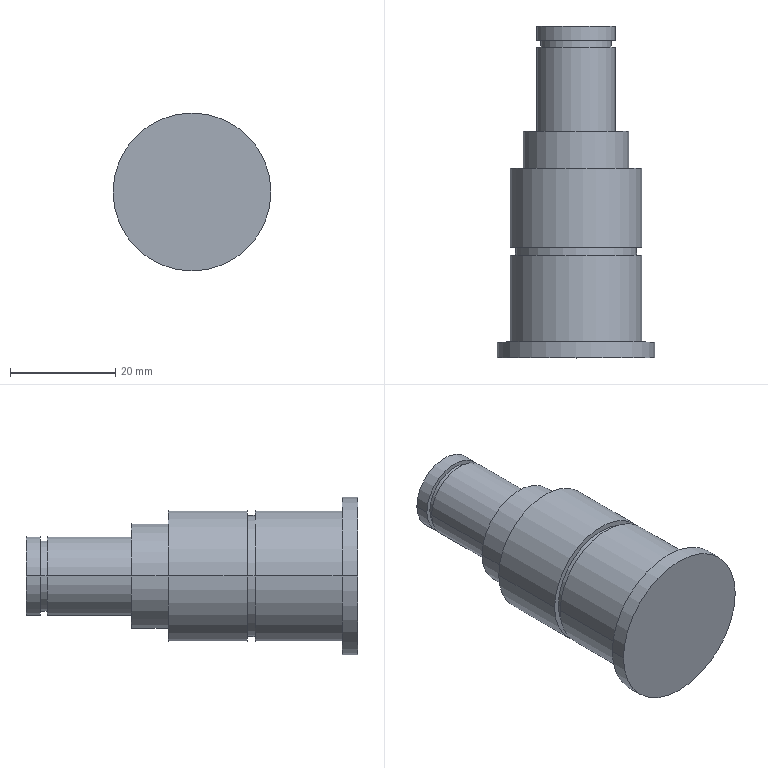Part | SolidWorks | features Revolution 1 | 1 solid | 25 faces | box 30 x 63 x 30 mm | volume 23893 mm3 | cylinder 16 | plane 9 | commonest cylinder face diameters 15 x4 25 x4 13.4 x2 20 x2 23 x2 30 x2
STEP:
#1=CARTESIAN_POINT('',(6.7,63.005,0.));
#2=VERTEX_POINT('',#1);
#3=CARTESIAN_POINT('',(-6.7,63.005,0.));
#4=VERTEX_POINT('',#3);
#5=CARTESIAN_POINT('',(0.,63.005,0.));
#6=DIRECTION('',(0.,-1.,0.));
#7=DIRECTION('',(1.,0.,0.));
#8=AXIS2_PLACEMENT_3D('',#5,#6,#7);
#9=CIRCLE('',#8,6.7);
#10=EDGE_CURVE('',#2,#4,#9,.T.);
#11=ORIENTED_EDGE('',*,*,#10,.T.);
#12=CARTESIAN_POINT('',(-6.7,61.705,0.));
#13=VERTEX_POINT('',#12);
#14=CARTESIAN_POINT('',(-6.7,65.705,0.));
#15=DIRECTION('',(0.,-1.,0.));
#16=VECTOR('',#15,1000.);
#17=LINE('',#14,#16);
#18=EDGE_CURVE('',#4,#13,#17,.T.);
#19=ORIENTED_EDGE('',*,*,#18,.T.);
#20=CARTESIAN_POINT('',(6.7,61.705,0.));
#21=VERTEX_POINT('',#20);
#22=CARTESIAN_POINT('',(0.,61.705,0.));
#23=DIRECTION('',(0.,-1.,0.));
#24=DIRECTION('',(1.,0.,0.));
#25=AXIS2_PLACEMENT_3D('',#22,#23,#24);
#26=CIRCLE('',#25,6.7);
#27=EDGE_CURVE('',#21,#13,#26,.T.);
#28=ORIENTED_EDGE('',*,*,#27,.F.);
#29=CARTESIAN_POINT('',(6.7,65.705,0.));
#30=DIRECTION('',(0.,-1.,0.));
#31=VECTOR('',#30,1000.);
#32=LINE('',#29,#31);
#33=EDGE_CURVE('',#2,#21,#32,.T.);
#34=ORIENTED_EDGE('',*,*,#33,.F.);
#35=EDGE_LOOP('',(#11,#19,#28,#34));
#36=FACE_OUTER_BOUND('',#35,.T.);
#37=CARTESIAN_POINT('',(0.,65.705,0.));
#38=DIRECTION('',(0.,-1.,0.));
#39=DIRECTION('',(1.,0.,0.));
#40=AXIS2_PLACEMENT_3D('',#37,#38,#39);
#41=CYLINDRICAL_SURFACE('',#40,6.7);
#42=ADVANCED_FACE('',(#36),#41,.T.);
#43=CARTESIAN_POINT('',(7.5,61.705,0.));
#44=VERTEX_POINT('',#43);
#45=CARTESIAN_POINT('',(-7.5,61.705,0.));
#46=VERTEX_POINT('',#45);
#47=CARTESIAN_POINT('',(0.,61.705,0.));
#48=DIRECTION('',(0.,-1.,0.));
#49=DIRECTION('',(1.,0.,0.));
#50=AXIS2_PLACEMENT_3D('',#47,#48,#49);
#51=CIRCLE('',#50,7.5);
#52=EDGE_CURVE('',#44,#46,#51,.T.);
#53=ORIENTED_EDGE('',*,*,#52,.T.);
#54=CARTESIAN_POINT('',(-7.5,45.705,0.));
#55=VERTEX_POINT('',#54);
#56=CARTESIAN_POINT('',(-7.5,65.705,0.));
#57=DIRECTION('',(0.,-1.,0.));
#58=VECTOR('',#57,1000.);
#59=LINE('',#56,#58);
#60=EDGE_CURVE('',#46,#55,#59,.T.);
#61=ORIENTED_EDGE('',*,*,#60,.T.);
#62=CARTESIAN_POINT('',(7.5,45.705,0.));
#63=VERTEX_POINT('',#62);
#64=CARTESIAN_POINT('',(0.,45.705,0.));
#65=DIRECTION('',(0.,-1.,0.));
#66=DIRECTION('',(1.,0.,0.));
#67=AXIS2_PLACEMENT_3D('',#64,#65,#66);
#68=CIRCLE('',#67,7.5);
#69=EDGE_CURVE('',#63,#55,#68,.T.);
#70=ORIENTED_EDGE('',*,*,#69,.F.);
#71=CARTESIAN_POINT('',(7.5,65.705,0.));
#72=DIRECTION('',(0.,-1.,0.));
#73=VECTOR('',#72,1000.);
#74=LINE('',#71,#73);
#75=EDGE_CURVE('',#44,#63,#74,.T.);
#76=ORIENTED_EDGE('',*,*,#75,.F.);
#77=EDGE_LOOP('',(#53,#61,#70,#76));
#78=FACE_OUTER_BOUND('',#77,.T.);
#79=CARTESIAN_POINT('',(0.,65.705,0.));
#80=DIRECTION('',(0.,-1.,0.));
#81=DIRECTION('',(1.,0.,0.));
#82=AXIS2_PLACEMENT_3D('',#79,#80,#81);
#83=CYLINDRICAL_SURFACE('',#82,7.5);
#84=ADVANCED_FACE('',(#78),#83,.T.);
#85=CARTESIAN_POINT('',(10.,45.705,0.));
#86=VERTEX_POINT('',#85);
#87=CARTESIAN_POINT('',(-10.,45.705,0.));
#88=VERTEX_POINT('',#87);
#89=CARTESIAN_POINT('',(0.,45.705,0.));
#90=DIRECTION('',(0.,-1.,0.));
#91=DIRECTION('',(1.,0.,0.));
#92=AXIS2_PLACEMENT_3D('',#89,#90,#91);
#93=CIRCLE('',#92,10.);
#94=EDGE_CURVE('',#86,#88,#93,.T.);
#95=ORIENTED_EDGE('',*,*,#94,.T.);
#96=CARTESIAN_POINT('',(-10.,38.705,0.));
#97=VERTEX_POINT('',#96);
#98=CARTESIAN_POINT('',(-10.,65.705,0.));
#99=DIRECTION('',(0.,-1.,0.));
#100=VECTOR('',#99,1000.);
#101=LINE('',#98,#100);
#102=EDGE_CURVE('',#88,#97,#101,.T.);
#103=ORIENTED_EDGE('',*,*,#102,.T.);
#104=CARTESIAN_POINT('',(10.,38.705,0.));
#105=VERTEX_POINT('',#104);
#106=CARTESIAN_POINT('',(0.,38.705,0.));
#107=DIRECTION('',(0.,-1.,0.));
#108=DIRECTION('',(1.,0.,0.));
#109=AXIS2_PLACEMENT_3D('',#106,#107,#108);
#110=CIRCLE('',#109,10.);
#111=EDGE_CURVE('',#105,#97,#110,.T.);
#112=ORIENTED_EDGE('',*,*,#111,.F.);
#113=CARTESIAN_POINT('',(10.,65.705,0.));
#114=DIRECTION('',(0.,-1.,0.));
#115=VECTOR('',#114,1000.);
#116=LINE('',#113,#115);
#117=EDGE_CURVE('',#86,#105,#116,.T.);
#118=ORIENTED_EDGE('',*,*,#117,.F.);
#119=EDGE_LOOP('',(#95,#103,#112,#118));
#120=FACE_OUTER_BOUND('',#119,.T.);
#121=CARTESIAN_POINT('',(0.,65.705,0.));
#122=DIRECTION('',(0.,-1.,0.));
#123=DIRECTION('',(1.,0.,0.));
#124=AXIS2_PLACEMENT_3D('',#121,#122,#123);
#125=CYLINDRICAL_SURFACE('',#124,10.);
#126=ADVANCED_FACE('',(#120),#125,.T.);
#127=CARTESIAN_POINT('',(12.5,38.705,0.));
#128=VERTEX_POINT('',#127);
#129=CARTESIAN_POINT('',(-12.5,38.705,0.));
#130=VERTEX_POINT('',#129);
#131=CARTESIAN_POINT('',(0.,38.705,0.));
#132=DIRECTION('',(0.,-1.,0.));
#133=DIRECTION('',(1.,0.,0.));
#134=AXIS2_PLACEMENT_3D('',#131,#132,#133);
#135=CIRCLE('',#134,12.5);
#136=EDGE_CURVE('',#128,#130,#135,.T.);
#137=ORIENTED_EDGE('',*,*,#136,.T.);
#138=CARTESIAN_POINT('',(-12.5,23.705,0.));
#139=VERTEX_POINT('',#138);
#140=CARTESIAN_POINT('',(-12.5,65.705,0.));
#141=DIRECTION('',(0.,-1.,0.));
#142=VECTOR('',#141,1000.);
#143=LINE('',#140,#142);
#144=EDGE_CURVE('',#130,#139,#143,.T.);
#145=ORIENTED_EDGE('',*,*,#144,.T.);
#146=CARTESIAN_POINT('',(12.5,23.705,0.));
#147=VERTEX_POINT('',#146);
#148=CARTESIAN_POINT('',(0.,23.705,0.));
#149=DIRECTION('',(0.,-1.,0.));
#150=DIRECTION('',(1.,0.,0.));
#151=AXIS2_PLACEMENT_3D('',#148,#149,#150);
#152=CIRCLE('',#151,12.5);
#153=EDGE_CURVE('',#147,#139,#152,.T.);
#154=ORIENTED_EDGE('',*,*,#153,.F.);
#155=CARTESIAN_POINT('',(12.5,65.705,0.));
#156=DIRECTION('',(0.,-1.,0.));
#157=VECTOR('',#156,1000.);
#158=LINE('',#155,#157);
#159=EDGE_CURVE('',#128,#147,#158,.T.);
#160=ORIENTED_EDGE('',*,*,#159,.F.);
#161=EDGE_LOOP('',(#137,#145,#154,#160));
#162=FACE_OUTER_BOUND('',#161,.T.);
#163=CARTESIAN_POINT('',(0.,65.705,0.));
#164=DIRECTION('',(0.,-1.,0.));
#165=DIRECTION('',(1.,0.,0.));
#166=AXIS2_PLACEMENT_3D('',#163,#164,#165);
#167=CYLINDRICAL_SURFACE('',#166,12.5);
#168=ADVANCED_FACE('',(#162),#167,.T.);
#169=CARTESIAN_POINT('',(11.5,23.705,0.));
#170=VERTEX_POINT('',#169);
#171=CARTESIAN_POINT('',(-11.5,23.705,0.));
#172=VERTEX_POINT('',#171);
#173=CARTESIAN_POINT('',(0.,23.705,0.));
#174=DIRECTION('',(0.,-1.,0.));
#175=DIRECTION('',(1.,0.,0.));
#176=AXIS2_PLACEMENT_3D('',#173,#174,#175);
#177=CIRCLE('',#176,11.5);
#178=EDGE_CURVE('',#170,#172,#177,.T.);
#179=ORIENTED_EDGE('',*,*,#178,.T.);
#180=CARTESIAN_POINT('',(-11.5,22.205,0.));
#181=VERTEX_POINT('',#180);
#182=CARTESIAN_POINT('',(-11.5,65.705,0.));
#183=DIRECTION('',(0.,-1.,0.));
#184=VECTOR('',#183,1000.);
#185=LINE('',#182,#184);
#186=EDGE_CURVE('',#172,#181,#185,.T.);
#187=ORIENTED_EDGE('',*,*,#186,.T.);
#188=CARTESIAN_POINT('',(11.5,22.205,0.));
#189=VERTEX_POINT('',#188);
#190=CARTESIAN_POINT('',(0.,22.205,0.));
#191=DIRECTION('',(0.,-1.,0.));
#192=DIRECTION('',(1.,0.,0.));
#193=AXIS2_PLACEMENT_3D('',#190,#191,#192);
#194=CIRCLE('',#193,11.5);
#195=EDGE_CURVE('',#189,#181,#194,.T.);
#196=ORIENTED_EDGE('',*,*,#195,.F.);
#197=CARTESIAN_POINT('',(11.5,65.705,0.));
#198=DIRECTION('',(0.,-1.,0.));
#199=VECTOR('',#198,1000.);
#200=LINE('',#197,#199);
#201=EDGE_CURVE('',#170,#189,#200,.T.);
#202=ORIENTED_EDGE('',*,*,#201,.F.);
#203=EDGE_LOOP('',(#179,#187,#196,#202));
#204=FACE_OUTER_BOUND('',#203,.T.);
#205=CARTESIAN_POINT('',(0.,65.705,0.));
#206=DIRECTION('',(0.,-1.,0.));
#207=DIRECTION('',(1.,0.,0.));
#208=AXIS2_PLACEMENT_3D('',#205,#206,#207);
#209=CYLINDRICAL_SURFACE('',#208,11.5);
#210=ADVANCED_FACE('',(#204),#209,.T.);
#211=CARTESIAN_POINT('',(12.5,22.205,0.));
#212=VERTEX_POINT('',#211);
#213=CARTESIAN_POINT('',(-12.5,22.205,0.));
#214=VERTEX_POINT('',#213);
#215=CARTESIAN_POINT('',(0.,22.205,0.));
#216=DIRECTION('',(0.,-1.,0.));
#217=DIRECTION('',(1.,0.,0.));
#218=AXIS2_PLACEMENT_3D('',#215,#216,#217);
#219=CIRCLE('',#218,12.5);
#220=EDGE_CURVE('',#212,#214,#219,.T.);
#221=ORIENTED_EDGE('',*,*,#220,.T.);
#222=CARTESIAN_POINT('',(-12.5,5.705,0.));
#223=VERTEX_POINT('',#222);
#224=CARTESIAN_POINT('',(-12.5,65.705,0.));
#225=DIRECTION('',(0.,-1.,0.));
#226=VECTOR('',#225,1000.);
#227=LINE('',#224,#226);
#228=EDGE_CURVE('',#214,#223,#227,.T.);
#229=ORIENTED_EDGE('',*,*,#228,.T.);
#230=CARTESIAN_POINT('',(12.5,5.705,0.));
#231=VERTEX_POINT('',#230);
#232=CARTESIAN_POINT('',(0.,5.705,0.));
#233=DIRECTION('',(0.,-1.,0.));
#234=DIRECTION('',(1.,0.,0.));
#235=AXIS2_PLACEMENT_3D('',#232,#233,#234);
#236=CIRCLE('',#235,12.5);
#237=EDGE_CURVE('',#231,#223,#236,.T.);
#238=ORIENTED_EDGE('',*,*,#237,.F.);
#239=CARTESIAN_POINT('',(12.5,65.705,0.));
#240=DIRECTION('',(0.,-1.,0.));
#241=VECTOR('',#240,1000.);
#242=LINE('',#239,#241);
#243=EDGE_CURVE('',#212,#231,#242,.T.);
#244=ORIENTED_EDGE('',*,*,#243,.F.);
#245=EDGE_LOOP('',(#221,#229,#238,#244));
#246=FACE_OUTER_BOUND('',#245,.T.);
#247=CARTESIAN_POINT('',(0.,65.705,0.));
#248=DIRECTION('',(0.,-1.,0.));
#249=DIRECTION('',(1.,0.,0.));
#250=AXIS2_PLACEMENT_3D('',#247,#248,#249);
#251=CYLINDRICAL_SURFACE('',#250,12.5);
#252=ADVANCED_FACE('',(#246),#251,.T.);
#253=CARTESIAN_POINT('',(15.,5.705,0.));
#254=VERTEX_POINT('',#253);
#255=CARTESIAN_POINT('',(-15.,5.705,0.));
#256=VERTEX_POINT('',#255);
#257=CARTESIAN_POINT('',(0.,5.705,0.));
#258=DIRECTION('',(0.,-1.,0.));
#259=DIRECTION('',(1.,0.,0.));
#260=AXIS2_PLACEMENT_3D('',#257,#258,#259);
#261=CIRCLE('',#260,15.);
#262=EDGE_CURVE('',#254,#256,#261,.T.);
#263=ORIENTED_EDGE('',*,*,#262,.T.);
#264=CARTESIAN_POINT('',(-15.,2.705,0.));
#265=VERTEX_POINT('',#264);
#266=CARTESIAN_POINT('',(-15.,65.705,0.));
#267=DIRECTION('',(0.,-1.,0.));
#268=VECTOR('',#267,1000.);
#269=LINE('',#266,#268);
#270=EDGE_CURVE('',#256,#265,#269,.T.);
#271=ORIENTED_EDGE('',*,*,#270,.T.);
#272=CARTESIAN_POINT('',(15.,2.705,0.));
#273=VERTEX_POINT('',#272);
#274=CARTESIAN_POINT('',(0.,2.705,0.));
#275=DIRECTION('',(0.,-1.,0.));
#276=DIRECTION('',(1.,0.,0.));
#277=AXIS2_PLACEMENT_3D('',#274,#275,#276);
#278=CIRCLE('',#277,15.);
#279=EDGE_CURVE('',#273,#265,#278,.T.);
#280=ORIENTED_EDGE('',*,*,#279,.F.);
#281=CARTESIAN_POINT('',(15.,65.705,0.));
#282=DIRECTION('',(0.,-1.,0.));
#283=VECTOR('',#282,1000.);
#284=LINE('',#281,#283);
#285=EDGE_CURVE('',#254,#273,#284,.T.);
#286=ORIENTED_EDGE('',*,*,#285,.F.);
#287=EDGE_LOOP('',(#263,#271,#280,#286));
#288=FACE_OUTER_BOUND('',#287,.T.);
#289=CARTESIAN_POINT('',(0.,65.705,0.));
#290=DIRECTION('',(0.,-1.,0.));
#291=DIRECTION('',(1.,0.,0.));
#292=AXIS2_PLACEMENT_3D('',#289,#290,#291);
#293=CYLINDRICAL_SURFACE('',#292,15.);
#294=ADVANCED_FACE('',(#288),#293,.T.);
#295=CARTESIAN_POINT('',(7.5,65.705,0.));
#296=VERTEX_POINT('',#295);
#297=CARTESIAN_POINT('',(-7.5,65.705,0.));
#298=VERTEX_POINT('',#297);
#299=CARTESIAN_POINT('',(0.,65.705,0.));
#300=DIRECTION('',(0.,-1.,0.));
#301=DIRECTION('',(1.,0.,0.));
#302=AXIS2_PLACEMENT_3D('',#299,#300,#301);
#303=CIRCLE('',#302,7.5);
#304=EDGE_CURVE('',#296,#298,#303,.T.);
#305=ORIENTED_EDGE('',*,*,#304,.T.);
#306=CARTESIAN_POINT('',(-7.5,63.005,0.));
#307=VERTEX_POINT('',#306);
#308=CARTESIAN_POINT('',(-7.5,65.705,0.));
#309=DIRECTION('',(0.,-1.,0.));
#310=VECTOR('',#309,1000.);
#311=LINE('',#308,#310);
#312=EDGE_CURVE('',#298,#307,#311,.T.);
#313=ORIENTED_EDGE('',*,*,#312,.T.);
#314=CARTESIAN_POINT('',(7.5,63.005,0.));
#315=VERTEX_POINT('',#314);
#316=CARTESIAN_POINT('',(0.,63.005,0.));
#317=DIRECTION('',(0.,-1.,0.));
#318=DIRECTION('',(1.,0.,0.));
#319=AXIS2_PLACEMENT_3D('',#316,#317,#318);
#320=CIRCLE('',#319,7.5);
#321=EDGE_CURVE('',#315,#307,#320,.T.);
#322=ORIENTED_EDGE('',*,*,#321,.F.);
#323=CARTESIAN_POINT('',(7.5,65.705,0.));
#324=DIRECTION('',(0.,-1.,0.));
#325=VECTOR('',#324,1000.);
#326=LINE('',#323,#325);
#327=EDGE_CURVE('',#296,#315,#326,.T.);
#328=ORIENTED_EDGE('',*,*,#327,.F.);
#329=EDGE_LOOP('',(#305,#313,#322,#328));
#330=FACE_OUTER_BOUND('',#329,.T.);
#331=CARTESIAN_POINT('',(0.,65.705,0.));
#332=DIRECTION('',(0.,-1.,0.));
#333=DIRECTION('',(1.,0.,0.));
#334=AXIS2_PLACEMENT_3D('',#331,#332,#333);
#335=CYLINDRICAL_SURFACE('',#334,7.5);
#336=ADVANCED_FACE('',(#330),#335,.T.);
#337=ORIENTED_EDGE('',*,*,#312,.F.);
#338=CARTESIAN_POINT('',(0.,65.705,0.));
#339=DIRECTION('',(0.,-1.,0.));
#340=DIRECTION('',(1.,0.,0.));
#341=AXIS2_PLACEMENT_3D('',#338,#339,#340);
#342=CIRCLE('',#341,7.5);
#343=EDGE_CURVE('',#298,#296,#342,.T.);
#344=ORIENTED_EDGE('',*,*,#343,.T.);
#345=ORIENTED_EDGE('',*,*,#327,.T.);
#346=CARTESIAN_POINT('',(0.,63.005,0.));
#347=DIRECTION('',(0.,-1.,0.));
#348=DIRECTION('',(1.,0.,0.));
#349=AXIS2_PLACEMENT_3D('',#346,#347,#348);
#350=CIRCLE('',#349,7.5);
#351=EDGE_CURVE('',#307,#315,#350,.T.);
#352=ORIENTED_EDGE('',*,*,#351,.F.);
#353=EDGE_LOOP('',(#337,#344,#345,#352));
#354=FACE_OUTER_BOUND('',#353,.T.);
#355=CARTESIAN_POINT('',(0.,65.705,0.));
#356=DIRECTION('',(0.,-1.,0.));
#357=DIRECTION('',(1.,0.,0.));
#358=AXIS2_PLACEMENT_3D('',#355,#356,#357);
#359=CYLINDRICAL_SURFACE('',#358,7.5);
#360=ADVANCED_FACE('',(#354),#359,.T.);
#361=ORIENTED_EDGE('',*,*,#304,.F.);
#362=ORIENTED_EDGE('',*,*,#343,.F.);
#363=EDGE_LOOP('',(#361,#362));
#364=FACE_OUTER_BOUND('',#363,.T.);
#365=CARTESIAN_POINT('',(7.5,65.705,0.));
#366=DIRECTION('',(0.,1.,0.));
#367=DIRECTION('',(-1.,0.,0.));
#368=AXIS2_PLACEMENT_3D('',#365,#366,#367);
#369=PLANE('',#368);
#370=ADVANCED_FACE('',(#364),#369,.T.);
#371=ORIENTED_EDGE('',*,*,#279,.T.);
#372=CARTESIAN_POINT('',(0.,2.705,0.));
#373=DIRECTION('',(0.,-1.,0.));
#374=DIRECTION('',(1.,0.,0.));
#375=AXIS2_PLACEMENT_3D('',#372,#373,#374);
#376=CIRCLE('',#375,15.);
#377=EDGE_CURVE('',#265,#273,#376,.T.);
#378=ORIENTED_EDGE('',*,*,#377,.T.);
#379=EDGE_LOOP('',(#371,#378));
#380=FACE_OUTER_BOUND('',#379,.T.);
#381=CARTESIAN_POINT('',(0.,2.705,0.));
#382=DIRECTION('',(0.,-1.,0.));
#383=DIRECTION('',(1.,0.,0.));
#384=AXIS2_PLACEMENT_3D('',#381,#382,#383);
#385=PLANE('',#384);
#386=ADVANCED_FACE('',(#380),#385,.T.);
#387=ORIENTED_EDGE('',*,*,#270,.F.);
#388=CARTESIAN_POINT('',(0.,5.705,0.));
#389=DIRECTION('',(0.,-1.,0.));
#390=DIRECTION('',(1.,0.,0.));
#391=AXIS2_PLACEMENT_3D('',#388,#389,#390);
#392=CIRCLE('',#391,15.);
#393=EDGE_CURVE('',#256,#254,#392,.T.);
#394=ORIENTED_EDGE('',*,*,#393,.T.);
#395=ORIENTED_EDGE('',*,*,#285,.T.);
#396=ORIENTED_EDGE('',*,*,#377,.F.);
#397=EDGE_LOOP('',(#387,#394,#395,#396));
#398=FACE_OUTER_BOUND('',#397,.T.);
#399=CARTESIAN_POINT('',(0.,65.705,0.));
#400=DIRECTION('',(0.,-1.,0.));
#401=DIRECTION('',(1.,0.,0.));
#402=AXIS2_PLACEMENT_3D('',#399,#400,#401);
#403=CYLINDRICAL_SURFACE('',#402,15.);
#404=ADVANCED_FACE('',(#398),#403,.T.);
#405=ORIENTED_EDGE('',*,*,#237,.T.);
#406=CARTESIAN_POINT('',(0.,5.705,0.));
#407=DIRECTION('',(0.,-1.,0.));
#408=DIRECTION('',(1.,0.,0.));
#409=AXIS2_PLACEMENT_3D('',#406,#407,#408);
#410=CIRCLE('',#409,12.5);
#411=EDGE_CURVE('',#223,#231,#410,.T.);
#412=ORIENTED_EDGE('',*,*,#411,.T.);
#413=EDGE_LOOP('',(#405,#412));
#414=FACE_BOUND('',#413,.T.);
#415=ORIENTED_EDGE('',*,*,#262,.F.);
#416=ORIENTED_EDGE('',*,*,#393,.F.);
#417=EDGE_LOOP('',(#415,#416));
#418=FACE_OUTER_BOUND('',#417,.T.);
#419=CARTESIAN_POINT('',(15.,5.705,0.));
#420=DIRECTION('',(0.,1.,0.));
#421=DIRECTION('',(-1.,0.,0.));
#422=AXIS2_PLACEMENT_3D('',#419,#420,#421);
#423=PLANE('',#422);
#424=ADVANCED_FACE('',(#414,#418),#423,.T.);
#425=ORIENTED_EDGE('',*,*,#228,.F.);
#426=CARTESIAN_POINT('',(0.,22.205,0.));
#427=DIRECTION('',(0.,-1.,0.));
#428=DIRECTION('',(1.,0.,0.));
#429=AXIS2_PLACEMENT_3D('',#426,#427,#428);
#430=CIRCLE('',#429,12.5);
#431=EDGE_CURVE('',#214,#212,#430,.T.);
#432=ORIENTED_EDGE('',*,*,#431,.T.);
#433=ORIENTED_EDGE('',*,*,#243,.T.);
#434=ORIENTED_EDGE('',*,*,#411,.F.);
#435=EDGE_LOOP('',(#425,#432,#433,#434));
#436=FACE_OUTER_BOUND('',#435,.T.);
#437=CARTESIAN_POINT('',(0.,65.705,0.));
#438=DIRECTION('',(0.,-1.,0.));
#439=DIRECTION('',(1.,0.,0.));
#440=AXIS2_PLACEMENT_3D('',#437,#438,#439);
#441=CYLINDRICAL_SURFACE('',#440,12.5);
#442=ADVANCED_FACE('',(#436),#441,.T.);
#443=ORIENTED_EDGE('',*,*,#195,.T.);
#444=CARTESIAN_POINT('',(0.,22.205,0.));
#445=DIRECTION('',(0.,-1.,0.));
#446=DIRECTION('',(1.,0.,0.));
#447=AXIS2_PLACEMENT_3D('',#444,#445,#446);
#448=CIRCLE('',#447,11.5);
#449=EDGE_CURVE('',#181,#189,#448,.T.);
#450=ORIENTED_EDGE('',*,*,#449,.T.);
#451=EDGE_LOOP('',(#443,#450));
#452=FACE_BOUND('',#451,.T.);
#453=ORIENTED_EDGE('',*,*,#220,.F.);
#454=ORIENTED_EDGE('',*,*,#431,.F.);
#455=EDGE_LOOP('',(#453,#454));
#456=FACE_OUTER_BOUND('',#455,.T.);
#457=CARTESIAN_POINT('',(12.5,22.205,0.));
#458=DIRECTION('',(0.,1.,0.));
#459=DIRECTION('',(-1.,0.,0.));
#460=AXIS2_PLACEMENT_3D('',#457,#458,#459);
#461=PLANE('',#460);
#462=ADVANCED_FACE('',(#452,#456),#461,.T.);
#463=ORIENTED_EDGE('',*,*,#186,.F.);
#464=CARTESIAN_POINT('',(0.,23.705,0.));
#465=DIRECTION('',(0.,-1.,0.));
#466=DIRECTION('',(1.,0.,0.));
#467=AXIS2_PLACEMENT_3D('',#464,#465,#466);
#468=CIRCLE('',#467,11.5);
#469=EDGE_CURVE('',#172,#170,#468,.T.);
#470=ORIENTED_EDGE('',*,*,#469,.T.);
#471=ORIENTED_EDGE('',*,*,#201,.T.);
#472=ORIENTED_EDGE('',*,*,#449,.F.);
#473=EDGE_LOOP('',(#463,#470,#471,#472));
#474=FACE_OUTER_BOUND('',#473,.T.);
#475=CARTESIAN_POINT('',(0.,65.705,0.));
#476=DIRECTION('',(0.,-1.,0.));
#477=DIRECTION('',(1.,0.,0.));
#478=AXIS2_PLACEMENT_3D('',#475,#476,#477);
#479=CYLINDRICAL_SURFACE('',#478,11.5);
#480=ADVANCED_FACE('',(#474),#479,.T.);
#481=ORIENTED_EDGE('',*,*,#153,.T.);
#482=CARTESIAN_POINT('',(0.,23.705,0.));
#483=DIRECTION('',(0.,-1.,0.));
#484=DIRECTION('',(1.,0.,0.));
#485=AXIS2_PLACEMENT_3D('',#482,#483,#484);
#486=CIRCLE('',#485,12.5);
#487=EDGE_CURVE('',#139,#147,#486,.T.);
#488=ORIENTED_EDGE('',*,*,#487,.T.);
#489=EDGE_LOOP('',(#481,#488));
#490=FACE_OUTER_BOUND('',#489,.T.);
#491=ORIENTED_EDGE('',*,*,#178,.F.);
#492=ORIENTED_EDGE('',*,*,#469,.F.);
#493=EDGE_LOOP('',(#491,#492));
#494=FACE_BOUND('',#493,.T.);
#495=CARTESIAN_POINT('',(11.5,23.705,0.));
#496=DIRECTION('',(0.,-1.,0.));
#497=DIRECTION('',(1.,0.,0.));
#498=AXIS2_PLACEMENT_3D('',#495,#496,#497);
#499=PLANE('',#498);
#500=ADVANCED_FACE('',(#490,#494),#499,.T.);
#501=ORIENTED_EDGE('',*,*,#144,.F.);
#502=CARTESIAN_POINT('',(0.,38.705,0.));
#503=DIRECTION('',(0.,-1.,0.));
#504=DIRECTION('',(1.,0.,0.));
#505=AXIS2_PLACEMENT_3D('',#502,#503,#504);
#506=CIRCLE('',#505,12.5);
#507=EDGE_CURVE('',#130,#128,#506,.T.);
#508=ORIENTED_EDGE('',*,*,#507,.T.);
#509=ORIENTED_EDGE('',*,*,#159,.T.);
#510=ORIENTED_EDGE('',*,*,#487,.F.);
#511=EDGE_LOOP('',(#501,#508,#509,#510));
#512=FACE_OUTER_BOUND('',#511,.T.);
#513=CARTESIAN_POINT('',(0.,65.705,0.));
#514=DIRECTION('',(0.,-1.,0.));
#515=DIRECTION('',(1.,0.,0.));
#516=AXIS2_PLACEMENT_3D('',#513,#514,#515);
#517=CYLINDRICAL_SURFACE('',#516,12.5);
#518=ADVANCED_FACE('',(#512),#517,.T.);
#519=ORIENTED_EDGE('',*,*,#111,.T.);
#520=CARTESIAN_POINT('',(0.,38.705,0.));
#521=DIRECTION('',(0.,-1.,0.));
#522=DIRECTION('',(1.,0.,0.));
#523=AXIS2_PLACEMENT_3D('',#520,#521,#522);
#524=CIRCLE('',#523,10.);
#525=EDGE_CURVE('',#97,#105,#524,.T.);
#526=ORIENTED_EDGE('',*,*,#525,.T.);
#527=EDGE_LOOP('',(#519,#526));
#528=FACE_BOUND('',#527,.T.);
#529=ORIENTED_EDGE('',*,*,#136,.F.);
#530=ORIENTED_EDGE('',*,*,#507,.F.);
#531=EDGE_LOOP('',(#529,#530));
#532=FACE_OUTER_BOUND('',#531,.T.);
#533=CARTESIAN_POINT('',(12.5,38.705,0.));
#534=DIRECTION('',(0.,1.,0.));
#535=DIRECTION('',(-1.,0.,0.));
#536=AXIS2_PLACEMENT_3D('',#533,#534,#535);
#537=PLANE('',#536);
#538=ADVANCED_FACE('',(#528,#532),#537,.T.);
#539=ORIENTED_EDGE('',*,*,#102,.F.);
#540=CARTESIAN_POINT('',(0.,45.705,0.));
#541=DIRECTION('',(0.,-1.,0.));
#542=DIRECTION('',(1.,0.,0.));
#543=AXIS2_PLACEMENT_3D('',#540,#541,#542);
#544=CIRCLE('',#543,10.);
#545=EDGE_CURVE('',#88,#86,#544,.T.);
#546=ORIENTED_EDGE('',*,*,#545,.T.);
#547=ORIENTED_EDGE('',*,*,#117,.T.);
#548=ORIENTED_EDGE('',*,*,#525,.F.);
#549=EDGE_LOOP('',(#539,#546,#547,#548));
#550=FACE_OUTER_BOUND('',#549,.T.);
#551=CARTESIAN_POINT('',(0.,65.705,0.));
#552=DIRECTION('',(0.,-1.,0.));
#553=DIRECTION('',(1.,0.,0.));
#554=AXIS2_PLACEMENT_3D('',#551,#552,#553);
#555=CYLINDRICAL_SURFACE('',#554,10.);
#556=ADVANCED_FACE('',(#550),#555,.T.);
#557=ORIENTED_EDGE('',*,*,#69,.T.);
#558=CARTESIAN_POINT('',(0.,45.705,0.));
#559=DIRECTION('',(0.,-1.,0.));
#560=DIRECTION('',(1.,0.,0.));
#561=AXIS2_PLACEMENT_3D('',#558,#559,#560);
#562=CIRCLE('',#561,7.5);
#563=EDGE_CURVE('',#55,#63,#562,.T.);
#564=ORIENTED_EDGE('',*,*,#563,.T.);
#565=EDGE_LOOP('',(#557,#564));
#566=FACE_BOUND('',#565,.T.);
#567=ORIENTED_EDGE('',*,*,#94,.F.);
#568=ORIENTED_EDGE('',*,*,#545,.F.);
#569=EDGE_LOOP('',(#567,#568));
#570=FACE_OUTER_BOUND('',#569,.T.);
#571=CARTESIAN_POINT('',(10.,45.705,0.));
#572=DIRECTION('',(0.,1.,0.));
#573=DIRECTION('',(-1.,0.,0.));
#574=AXIS2_PLACEMENT_3D('',#571,#572,#573);
#575=PLANE('',#574);
#576=ADVANCED_FACE('',(#566,#570),#575,.T.);
#577=ORIENTED_EDGE('',*,*,#60,.F.);
#578=CARTESIAN_POINT('',(0.,61.705,0.));
#579=DIRECTION('',(0.,-1.,0.));
#580=DIRECTION('',(1.,0.,0.));
#581=AXIS2_PLACEMENT_3D('',#578,#579,#580);
#582=CIRCLE('',#581,7.5);
#583=EDGE_CURVE('',#46,#44,#582,.T.);
#584=ORIENTED_EDGE('',*,*,#583,.T.);
#585=ORIENTED_EDGE('',*,*,#75,.T.);
#586=ORIENTED_EDGE('',*,*,#563,.F.);
#587=EDGE_LOOP('',(#577,#584,#585,#586));
#588=FACE_OUTER_BOUND('',#587,.T.);
#589=CARTESIAN_POINT('',(0.,65.705,0.));
#590=DIRECTION('',(0.,-1.,0.));
#591=DIRECTION('',(1.,0.,0.));
#592=AXIS2_PLACEMENT_3D('',#589,#590,#591);
#593=CYLINDRICAL_SURFACE('',#592,7.5);
#594=ADVANCED_FACE('',(#588),#593,.T.);
#595=ORIENTED_EDGE('',*,*,#27,.T.);
#596=CARTESIAN_POINT('',(0.,61.705,0.));
#597=DIRECTION('',(0.,-1.,0.));
#598=DIRECTION('',(1.,0.,0.));
#599=AXIS2_PLACEMENT_3D('',#596,#597,#598);
#600=CIRCLE('',#599,6.7);
#601=EDGE_CURVE('',#13,#21,#600,.T.);
#602=ORIENTED_EDGE('',*,*,#601,.T.);
#603=EDGE_LOOP('',(#595,#602));
#604=FACE_BOUND('',#603,.T.);
#605=ORIENTED_EDGE('',*,*,#52,.F.);
#606=ORIENTED_EDGE('',*,*,#583,.F.);
#607=EDGE_LOOP('',(#605,#606));
#608=FACE_OUTER_BOUND('',#607,.T.);
#609=CARTESIAN_POINT('',(7.5,61.705,0.));
#610=DIRECTION('',(0.,1.,0.));
#611=DIRECTION('',(-1.,0.,0.));
#612=AXIS2_PLACEMENT_3D('',#609,#610,#611);
#613=PLANE('',#612);
#614=ADVANCED_FACE('',(#604,#608),#613,.T.);
#615=ORIENTED_EDGE('',*,*,#18,.F.);
#616=CARTESIAN_POINT('',(0.,63.005,0.));
#617=DIRECTION('',(0.,-1.,0.));
#618=DIRECTION('',(1.,0.,0.));
#619=AXIS2_PLACEMENT_3D('',#616,#617,#618);
#620=CIRCLE('',#619,6.7);
#621=EDGE_CURVE('',#4,#2,#620,.T.);
#622=ORIENTED_EDGE('',*,*,#621,.T.);
#623=ORIENTED_EDGE('',*,*,#33,.T.);
#624=ORIENTED_EDGE('',*,*,#601,.F.);
#625=EDGE_LOOP('',(#615,#622,#623,#624));
#626=FACE_OUTER_BOUND('',#625,.T.);
#627=CARTESIAN_POINT('',(0.,65.705,0.));
#628=DIRECTION('',(0.,-1.,0.));
#629=DIRECTION('',(1.,0.,0.));
#630=AXIS2_PLACEMENT_3D('',#627,#628,#629);
#631=CYLINDRICAL_SURFACE('',#630,6.7);
#632=ADVANCED_FACE('',(#626),#631,.T.);
#633=ORIENTED_EDGE('',*,*,#321,.T.);
#634=ORIENTED_EDGE('',*,*,#351,.T.);
#635=EDGE_LOOP('',(#633,#634));
#636=FACE_OUTER_BOUND('',#635,.T.);
#637=ORIENTED_EDGE('',*,*,#10,.F.);
#638=ORIENTED_EDGE('',*,*,#621,.F.);
#639=EDGE_LOOP('',(#637,#638));
#640=FACE_BOUND('',#639,.T.);
#641=CARTESIAN_POINT('',(6.7,63.005,0.));
#642=DIRECTION('',(0.,-1.,0.));
#643=DIRECTION('',(1.,0.,0.));
#644=AXIS2_PLACEMENT_3D('',#641,#642,#643);
#645=PLANE('',#644);
#646=ADVANCED_FACE('',(#636,#640),#645,.T.);
#647=CLOSED_SHELL('',(#42,#84,#126,#168,#210,#252,#294,#336,#360,#370,#386,#404,#424,#442,#462,#480,#500,#518,#538,#556,#576,#594,#614,#632,#646));
#648=MANIFOLD_SOLID_BREP('',#647);
#649=CARTESIAN_POINT('',(0.,0.,0.));
#650=DIRECTION('',(0.,0.,1.));
#651=DIRECTION('',(1.,0.,0.));
#652=AXIS2_PLACEMENT_3D('',#649,#650,#651);
#653=(LENGTH_UNIT()NAMED_UNIT(*)SI_UNIT(.MILLI.,.METRE.));
#654=UNCERTAINTY_MEASURE_WITH_UNIT(LENGTH_MEASURE(0.00001),#653,'','');
#655=(NAMED_UNIT(*)PLANE_ANGLE_UNIT()SI_UNIT($,.RADIAN.));
#656=(NAMED_UNIT(*)SI_UNIT($,.STERADIAN.)SOLID_ANGLE_UNIT());
#657=(GEOMETRIC_REPRESENTATION_CONTEXT(3)GLOBAL_UNCERTAINTY_ASSIGNED_CONTEXT((#654))GLOBAL_UNIT_ASSIGNED_CONTEXT((#653,#655,#656))REPRESENTATION_CONTEXT('',''));
#658=ADVANCED_BREP_SHAPE_REPRESENTATION('',(#648,#652),#657);